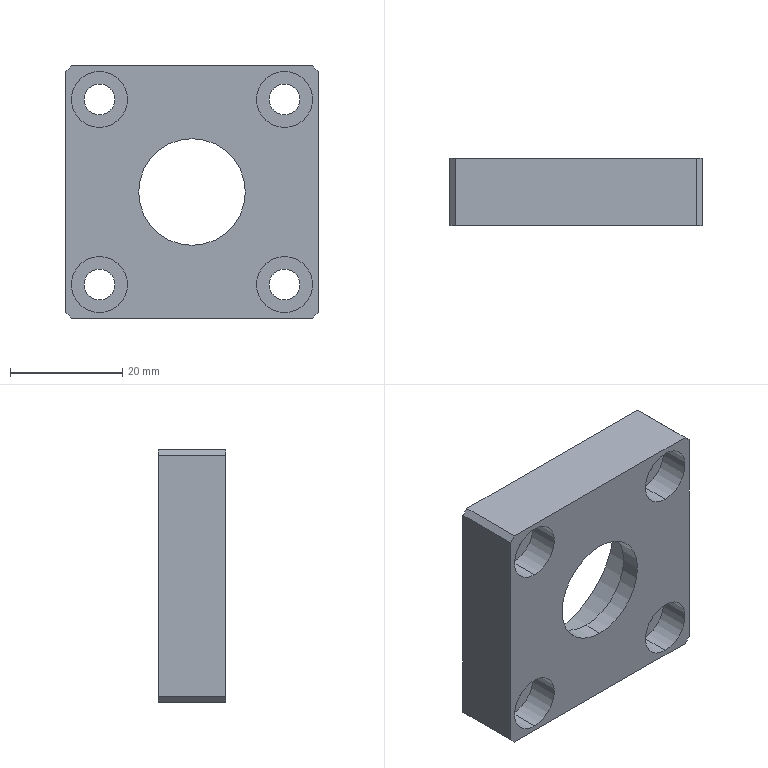Part | STEP file | PN_0055 | 1 solid | 35 faces | box 45 x 12 x 45 mm | volume 14544 mm3 | cylinder 20 | plane 15 | commonest cylinder face diameters 5.5 x8 10 x8 19 x2 31 x2